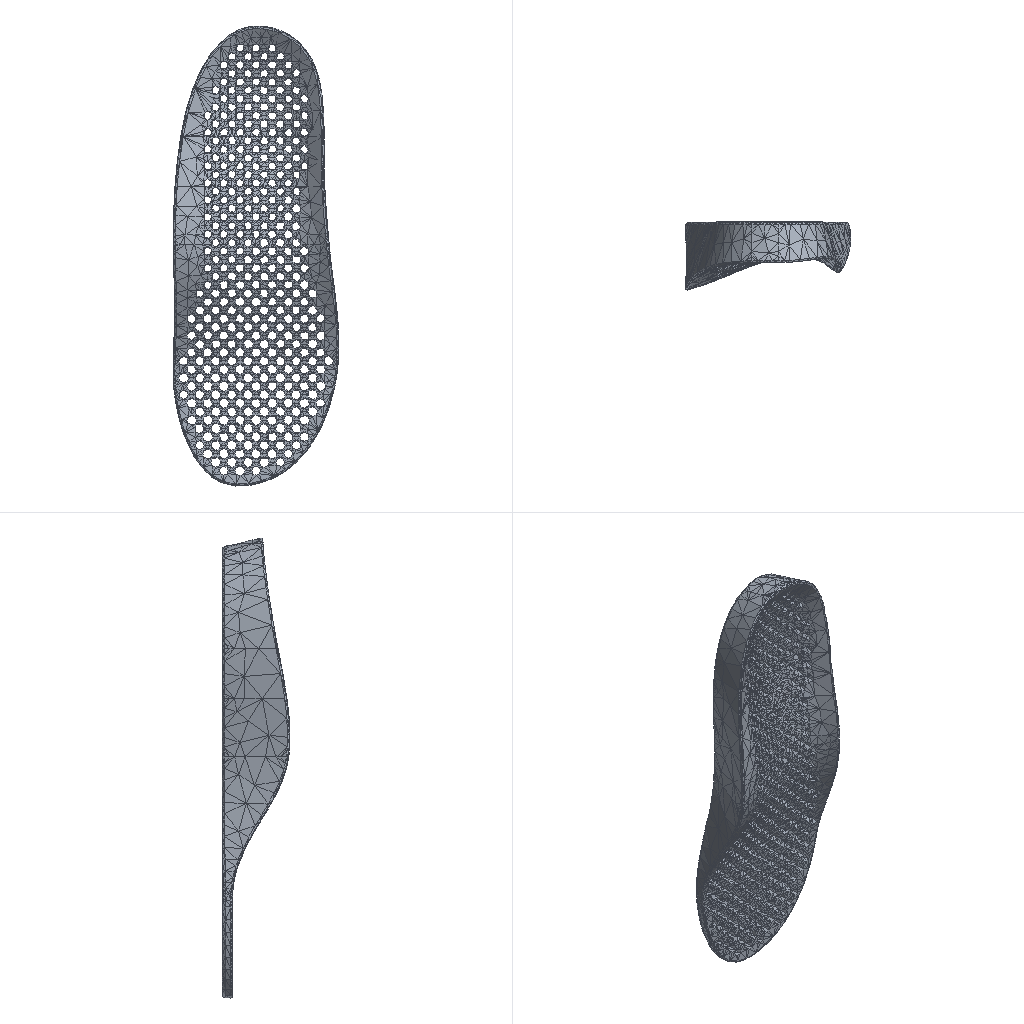Simulation study | ansys workbench
Set-up summary:
category,name,step,type,value,unit,region
solver,ansys_mapdl
solver,version,,,22.2
solver,version,,,22.2
solver,version,,,22.2
solver,version,,,22.2
units,MKS,,stated
analysis,deck1,,static,static
load_step,requested,,,1
analysis,nlgeom,,,False
mesh,nodes,,,61292
mesh,elements,,,33302
element_type,ANSYS 187 (type 1),,solid,29100
element_type,ANSYS 154 (type 2),,surface,4202
load,load commands in deck,,count,3
bc,support commands in deck,,count,1
named_set,_FIXEDSU,,component
analysis,deck2,,static,static
load_step,requested,,,1
analysis,nlgeom,,,False
mesh,nodes,,,233996
mesh,elements,,,130739
element_type,ANSYS 187 (type 1),,solid,117893
element_type,ANSYS 154 (type 2),,surface,12846
load,load commands in deck,,count,3
bc,support commands in deck,,count,1
named_set,_FIXEDSU,,component
analysis,deck3,,static,static
load_step,requested,,,1
analysis,nlgeom,,,False
mesh,nodes,,,233996
mesh,elements,,,130739
element_type,ANSYS 187 (type 1),,solid,117893
element_type,ANSYS 154 (type 2),,surface,12846
load,load commands in deck,,count,3
bc,support commands in deck,,count,1
named_set,_FIXEDSU,,component
analysis,deck4,,static,static
load_step,requested,,,1
analysis,nlgeom,,,False
mesh,nodes,,,61292
mesh,elements,,,33302
element_type,ANSYS 187 (type 1),,solid,29100
element_type,ANSYS 154 (type 2),,surface,4202
load,load commands in deck,,count,3
bc,support commands in deck,,count,1
named_set,_FIXEDSU,,component
material,1,,in results
material,1,,in results
material,1,,in results
material,1,,in results
check,setup vs results,,match,4202 surface effect element(s) are not in the reader's mesh and were not compared
check,setup vs results,,match,12846 surface effect element(s) are not in the reader's mesh and were not compared
check,setup vs results,,match,12846 surface effect element(s) are not in the reader's mesh and were not compared
check,setup vs results,,match,4202 surface effect element(s) are not in the reader's mesh and were not compared
Results summary:
result,analysis,,,static
result,last_loadstep,,,1
result,primary field,,,displacement
result,reaction total,1,FX,-0.0,N
result,reaction total,1,FY,-1200.001,N
result,reaction total,1,FZ,0.0,N
result,mass,,,0.2019,"MKS: m, kg, N, s, V, A, degC"
result,analysis,,,static
result,last_loadstep,,,1
result,primary field,,,displacement
result,reaction total,1,FX,-0.0,N
result,reaction total,1,FY,-350,N
result,reaction total,1,FZ,0.0,N
result,mass,,,0.1629,"MKS: m, kg, N, s, V, A, degC"
result,analysis,,,static
result,last_loadstep,,,1
result,primary field,,,displacement
result,reaction total,1,FX,-0.0,N
result,reaction total,1,FY,-1199.999,N
result,reaction total,1,FZ,0.0,N
result,mass,,,0.1629,"MKS: m, kg, N, s, V, A, degC"
result,analysis,,,static
result,last_loadstep,,,1
result,primary field,,,displacement
result,reaction total,1,FX,-0.0,N
result,reaction total,1,FY,-350,N
result,reaction total,1,FZ,0.0,N
result,mass,,,0.2019,"MKS: m, kg, N, s, V, A, degC"